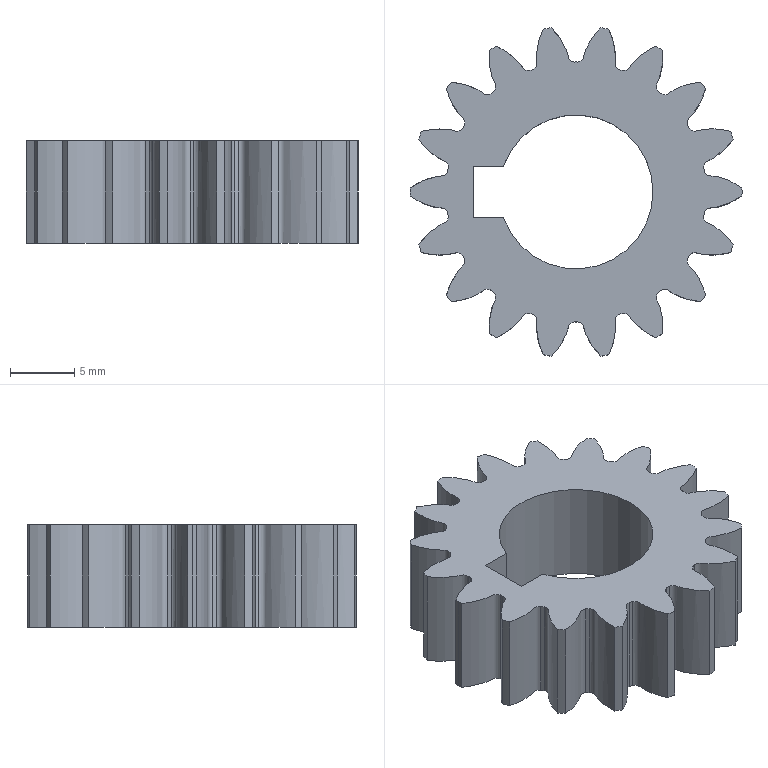Part | SolidWorks | features CirPattern 1, Cut 1, Extrusion 1, ICE 1, RefAxis 1 | 1 solid | 79 faces | box 25.875 x 25.587 x 8 mm | volume 2389 mm3 | cylinder 38 | spline 36 | plane 5 | commonest cylinder face diameters 25.875 x19 20.25 x18 12 x1